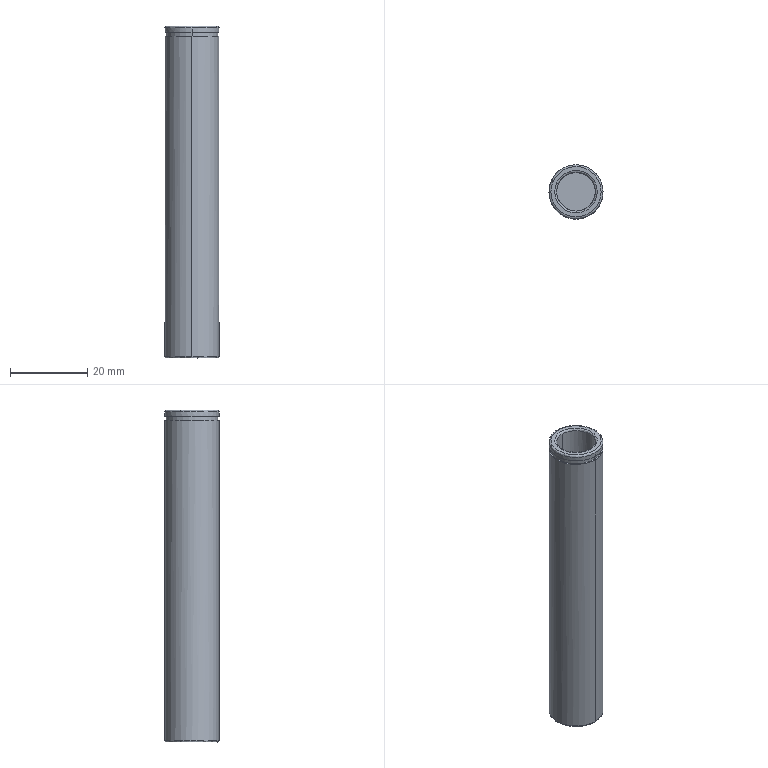Part | SolidWorks | features BaseBody 1 | 1 solid | 30 faces | box 14 x 14 x 86 mm | volume 10942 mm3 | cylinder 14 | spline 8 | plane 8 | commonest cylinder face diameters 10 x4 14 x4 4.2 x2 11.1 x2 13.4 x2
STEP:
#1=CARTESIAN_POINT('',(564.458,-176.727,213.045));
#2=VERTEX_POINT('',#1);
#3=CARTESIAN_POINT('',(552.284,-171.126,213.045));
#4=VERTEX_POINT('',#3);
#5=CARTESIAN_POINT('',(564.458,-176.727,213.045));
#6=CARTESIAN_POINT('',(570.058,-164.553,213.045));
#7=CARTESIAN_POINT('',(557.885,-158.953,213.045));
#8=CARTESIAN_POINT('',(552.284,-171.126,213.045));
#9=(BOUNDED_CURVE()B_SPLINE_CURVE(3,(#5,#6,#7,#8),.UNSPECIFIED.,.F.,.F.)B_SPLINE_CURVE_WITH_KNOTS((4,4),(0.,1.),.UNSPECIFIED.)CURVE()GEOMETRIC_REPRESENTATION_ITEM()RATIONAL_B_SPLINE_CURVE((1.,0.3333,0.3333,1.))REPRESENTATION_ITEM(''));
#10=EDGE_CURVE('',#2,#4,#9,.T.);
#11=ORIENTED_EDGE('',*,*,#10,.T.);
#12=CARTESIAN_POINT('',(552.012,-171.001,213.345));
#13=VERTEX_POINT('',#12);
#14=CARTESIAN_POINT('',(552.284,-171.126,213.345));
#15=DIRECTION('',(0.4179,0.9085,0.000000003));
#16=DIRECTION('',(-0.9085,0.4179,0.000000002));
#17=AXIS2_PLACEMENT_3D('',#14,#15,#16);
#18=CIRCLE('',#17,0.3);
#19=EDGE_CURVE('',#4,#13,#18,.T.);
#20=ORIENTED_EDGE('',*,*,#19,.T.);
#21=CARTESIAN_POINT('',(558.371,-166.927,213.345));
#22=VERTEX_POINT('',#21);
#23=CARTESIAN_POINT('',(558.371,-173.927,213.345));
#24=DIRECTION('',(0.000000001,-0.000000003,1.));
#25=DIRECTION('',(0.,1.,0.000000003));
#26=AXIS2_PLACEMENT_3D('',#23,#24,#25);
#27=CIRCLE('',#26,7.);
#28=EDGE_CURVE('',#22,#13,#27,.T.);
#29=ORIENTED_EDGE('',*,*,#28,.F.);
#30=CARTESIAN_POINT('',(564.73,-176.852,213.345));
#31=VERTEX_POINT('',#30);
#32=CARTESIAN_POINT('',(558.371,-173.927,213.345));
#33=DIRECTION('',(0.000000001,-0.000000003,1.));
#34=DIRECTION('',(0.,1.,0.000000003));
#35=AXIS2_PLACEMENT_3D('',#32,#33,#34);
#36=CIRCLE('',#35,7.);
#37=EDGE_CURVE('',#31,#22,#36,.T.);
#38=ORIENTED_EDGE('',*,*,#37,.F.);
#39=CARTESIAN_POINT('',(564.458,-176.727,213.345));
#40=DIRECTION('',(-0.4179,-0.9085,-0.000000003));
#41=DIRECTION('',(0.9085,-0.4179,-0.000000002));
#42=AXIS2_PLACEMENT_3D('',#39,#40,#41);
#43=CIRCLE('',#42,0.3);
#44=EDGE_CURVE('',#2,#31,#43,.T.);
#45=ORIENTED_EDGE('',*,*,#44,.F.);
#46=EDGE_LOOP('',(#11,#20,#29,#38,#45));
#47=FACE_OUTER_BOUND('',#46,.T.);
#48=CARTESIAN_POINT('',(552.284,-171.126,213.045));
#49=CARTESIAN_POINT('',(557.885,-158.953,213.045));
#50=CARTESIAN_POINT('',(570.058,-164.553,213.045));
#51=CARTESIAN_POINT('',(564.458,-176.727,213.045));
#52=CARTESIAN_POINT('',(552.125,-171.053,213.045));
#53=CARTESIAN_POINT('',(557.872,-158.56,213.045));
#54=CARTESIAN_POINT('',(570.365,-164.307,213.045));
#55=CARTESIAN_POINT('',(564.617,-176.8,213.045));
#56=CARTESIAN_POINT('',(552.012,-171.001,213.169));
#57=CARTESIAN_POINT('',(557.863,-158.282,213.169));
#58=CARTESIAN_POINT('',(570.581,-164.134,213.169));
#59=CARTESIAN_POINT('',(564.73,-176.852,213.169));
#60=CARTESIAN_POINT('',(552.012,-171.001,213.345));
#61=CARTESIAN_POINT('',(557.863,-158.282,213.345));
#62=CARTESIAN_POINT('',(570.581,-164.134,213.345));
#63=CARTESIAN_POINT('',(564.73,-176.852,213.345));
#64=(BOUNDED_SURFACE()B_SPLINE_SURFACE(3,3,((#48,#49,#50,#51),(#52,#53,#54,#55),(#56,#57,#58,#59),(#60,#61,#62,#63)),.UNSPECIFIED.,.F.,.F.,.F.)B_SPLINE_SURFACE_WITH_KNOTS((4,4),(4,4),(0.,1.),(0.,1.),.UNSPECIFIED.)GEOMETRIC_REPRESENTATION_ITEM()RATIONAL_B_SPLINE_SURFACE(((1.,0.3333,0.3333,1.),(0.8047,0.2682,0.2682,0.8047),(0.8047,0.2682,0.2682,0.8047),(1.,0.3333,0.3333,1.)))REPRESENTATION_ITEM('')SURFACE());
#65=ADVANCED_FACE('',(#47),#64,.T.);
#66=CARTESIAN_POINT('',(558.371,-176.027,213.345));
#67=VERTEX_POINT('',#66);
#68=CARTESIAN_POINT('',(560.279,-174.804,213.345));
#69=VERTEX_POINT('',#68);
#70=CARTESIAN_POINT('',(558.371,-173.927,213.345));
#71=DIRECTION('',(0.000000001,-0.000000003,1.));
#72=DIRECTION('',(-0.9085,0.4179,0.000000002));
#73=AXIS2_PLACEMENT_3D('',#70,#71,#72);
#74=CIRCLE('',#73,2.1);
#75=EDGE_CURVE('',#67,#69,#74,.T.);
#76=ORIENTED_EDGE('',*,*,#75,.T.);
#77=CARTESIAN_POINT('',(560.551,-174.93,213.045));
#78=VERTEX_POINT('',#77);
#79=CARTESIAN_POINT('',(560.551,-174.93,213.345));
#80=DIRECTION('',(-0.4179,-0.9085,-0.000000003));
#81=DIRECTION('',(0.9085,-0.4179,-0.000000002));
#82=AXIS2_PLACEMENT_3D('',#79,#80,#81);
#83=CIRCLE('',#82,0.3);
#84=EDGE_CURVE('',#69,#78,#83,.T.);
#85=ORIENTED_EDGE('',*,*,#84,.T.);
#86=CARTESIAN_POINT('',(556.191,-172.924,213.045));
#87=VERTEX_POINT('',#86);
#88=CARTESIAN_POINT('',(556.191,-172.924,213.045));
#89=CARTESIAN_POINT('',(556.127,-173.062,213.045));
#90=CARTESIAN_POINT('',(556.052,-173.275,213.045));
#91=CARTESIAN_POINT('',(556.001,-173.533,213.045));
#92=CARTESIAN_POINT('',(555.985,-173.664,213.045));
#93=CARTESIAN_POINT('',(555.98,-173.721,213.045));
#94=CARTESIAN_POINT('',(555.977,-173.758,213.045));
#95=CARTESIAN_POINT('',(555.976,-173.776,213.045));
#96=CARTESIAN_POINT('',(555.957,-174.127,213.045));
#97=CARTESIAN_POINT('',(556.005,-174.449,213.045));
#98=CARTESIAN_POINT('',(556.177,-174.914,213.045));
#99=CARTESIAN_POINT('',(556.285,-175.134,213.045));
#100=CARTESIAN_POINT('',(556.448,-175.367,213.045));
#101=CARTESIAN_POINT('',(556.539,-175.478,213.045));
#102=CARTESIAN_POINT('',(556.58,-175.524,213.045));
#103=CARTESIAN_POINT('',(556.607,-175.554,213.045));
#104=CARTESIAN_POINT('',(556.623,-175.571,213.045));
#105=CARTESIAN_POINT('',(556.846,-175.805,213.045));
#106=CARTESIAN_POINT('',(557.091,-175.979,213.045));
#107=CARTESIAN_POINT('',(557.506,-176.171,213.045));
#108=CARTESIAN_POINT('',(557.719,-176.245,213.045));
#109=CARTESIAN_POINT('',(557.977,-176.296,213.045));
#110=CARTESIAN_POINT('',(558.108,-176.313,213.045));
#111=CARTESIAN_POINT('',(558.165,-176.318,213.045));
#112=CARTESIAN_POINT('',(558.203,-176.321,213.045));
#113=CARTESIAN_POINT('',(558.22,-176.322,213.045));
#114=CARTESIAN_POINT('',(558.571,-176.341,213.045));
#115=CARTESIAN_POINT('',(558.893,-176.292,213.045));
#116=CARTESIAN_POINT('',(559.359,-176.12,213.045));
#117=CARTESIAN_POINT('',(559.578,-176.013,213.045));
#118=CARTESIAN_POINT('',(559.811,-175.85,213.045));
#119=CARTESIAN_POINT('',(559.922,-175.759,213.045));
#120=CARTESIAN_POINT('',(559.968,-175.718,213.045));
#121=CARTESIAN_POINT('',(559.999,-175.69,213.045));
#122=CARTESIAN_POINT('',(560.015,-175.675,213.045));
#123=CARTESIAN_POINT('',(560.25,-175.451,213.045));
#124=CARTESIAN_POINT('',(560.424,-175.207,213.045));
#125=CARTESIAN_POINT('',(560.551,-174.93,213.045));
#126=B_SPLINE_CURVE_WITH_KNOTS('',3,(#88,#89,#90,#91,#92,#93,#94,#95,#96,#97,#98,#99,#100,#101,#102,#103,#104,#105,#106,#107,#108,#109,#110,#111,#112,#113,#114,#115,#116,#117,#118,#119,#120,#121,#122,#123,#124,#125),.UNSPECIFIED.,.F.,.F.,(4,1,1,1,2,2,2,1,1,1,2,2,2,1,1,1,2,2,2,1,1,1,2,2,4),(0.,0.0625,0.09375,0.1094,0.1172,0.125,0.25,0.3125,0.3437,0.3594,0.3672,0.375,0.5,0.5625,0.5937,0.6094,0.6172,0.625,0.75,0.8125,0.8437,0.8594,0.8672,0.875,1.),.UNSPECIFIED.);
#127=EDGE_CURVE('',#87,#78,#126,.T.);
#128=ORIENTED_EDGE('',*,*,#127,.F.);
#129=CARTESIAN_POINT('',(556.463,-173.049,213.345));
#130=VERTEX_POINT('',#129);
#131=CARTESIAN_POINT('',(556.191,-172.924,213.345));
#132=DIRECTION('',(0.4179,0.9085,0.000000003));
#133=DIRECTION('',(-0.9085,0.4179,0.000000002));
#134=AXIS2_PLACEMENT_3D('',#131,#132,#133);
#135=CIRCLE('',#134,0.3);
#136=EDGE_CURVE('',#130,#87,#135,.T.);
#137=ORIENTED_EDGE('',*,*,#136,.F.);
#138=CARTESIAN_POINT('',(558.371,-173.927,213.345));
#139=DIRECTION('',(0.000000001,-0.000000003,1.));
#140=DIRECTION('',(-0.9085,0.4179,0.000000002));
#141=AXIS2_PLACEMENT_3D('',#138,#139,#140);
#142=CIRCLE('',#141,2.1);
#143=EDGE_CURVE('',#130,#67,#142,.T.);
#144=ORIENTED_EDGE('',*,*,#143,.T.);
#145=EDGE_LOOP('',(#76,#85,#128,#137,#144));
#146=FACE_OUTER_BOUND('',#145,.T.);
#147=CARTESIAN_POINT('',(560.279,-174.804,213.345));
#148=CARTESIAN_POINT('',(558.523,-178.62,213.345));
#149=CARTESIAN_POINT('',(554.708,-176.864,213.345));
#150=CARTESIAN_POINT('',(556.463,-173.049,213.345));
#151=CARTESIAN_POINT('',(560.279,-174.804,213.169));
#152=CARTESIAN_POINT('',(558.523,-178.62,213.169));
#153=CARTESIAN_POINT('',(554.708,-176.864,213.169));
#154=CARTESIAN_POINT('',(556.463,-173.049,213.169));
#155=CARTESIAN_POINT('',(560.392,-174.856,213.045));
#156=CARTESIAN_POINT('',(558.532,-178.898,213.045));
#157=CARTESIAN_POINT('',(554.491,-177.038,213.045));
#158=CARTESIAN_POINT('',(556.35,-172.997,213.045));
#159=CARTESIAN_POINT('',(560.551,-174.93,213.045));
#160=CARTESIAN_POINT('',(558.545,-179.29,213.045));
#161=CARTESIAN_POINT('',(554.185,-177.284,213.045));
#162=CARTESIAN_POINT('',(556.191,-172.924,213.045));
#163=(BOUNDED_SURFACE()B_SPLINE_SURFACE(3,3,((#147,#148,#149,#150),(#151,#152,#153,#154),(#155,#156,#157,#158),(#159,#160,#161,#162)),.UNSPECIFIED.,.F.,.F.,.F.)B_SPLINE_SURFACE_WITH_KNOTS((4,4),(4,4),(0.,1.),(0.,1.),.UNSPECIFIED.)GEOMETRIC_REPRESENTATION_ITEM()RATIONAL_B_SPLINE_SURFACE(((1.,0.3333,0.3333,1.),(0.8047,0.2682,0.2682,0.8047),(0.8047,0.2682,0.2682,0.8047),(1.,0.3333,0.3333,1.)))REPRESENTATION_ITEM('')SURFACE());
#164=ADVANCED_FACE('',(#146),#163,.T.);
#165=CARTESIAN_POINT('',(564.276,-176.643,299.045));
#166=VERTEX_POINT('',#165);
#167=CARTESIAN_POINT('',(552.466,-171.21,299.045));
#168=VERTEX_POINT('',#167);
#169=CARTESIAN_POINT('',(564.276,-176.643,299.045));
#170=CARTESIAN_POINT('',(558.843,-188.453,299.045));
#171=CARTESIAN_POINT('',(547.033,-183.02,299.045));
#172=CARTESIAN_POINT('',(552.466,-171.21,299.045));
#173=(BOUNDED_CURVE()B_SPLINE_CURVE(3,(#169,#170,#171,#172),.UNSPECIFIED.,.F.,.F.)B_SPLINE_CURVE_WITH_KNOTS((4,4),(0.,1.),.UNSPECIFIED.)CURVE()GEOMETRIC_REPRESENTATION_ITEM()RATIONAL_B_SPLINE_CURVE((1.,0.3333,0.3333,1.))REPRESENTATION_ITEM(''));
#174=EDGE_CURVE('',#166,#168,#173,.T.);
#175=ORIENTED_EDGE('',*,*,#174,.T.);
#176=CARTESIAN_POINT('',(552.012,-171.001,298.545));
#177=VERTEX_POINT('',#176);
#178=CARTESIAN_POINT('',(552.466,-171.21,298.545));
#179=DIRECTION('',(-0.4179,-0.9085,-0.000000003));
#180=DIRECTION('',(-0.9085,0.4179,0.000000002));
#181=AXIS2_PLACEMENT_3D('',#178,#179,#180);
#182=CIRCLE('',#181,0.5);
#183=EDGE_CURVE('',#168,#177,#182,.T.);
#184=ORIENTED_EDGE('',*,*,#183,.T.);
#185=CARTESIAN_POINT('',(558.371,-180.927,298.545));
#186=VERTEX_POINT('',#185);
#187=CARTESIAN_POINT('',(558.371,-173.927,298.545));
#188=DIRECTION('',(-0.000000001,0.000000003,-1.));
#189=DIRECTION('',(0.,1.,0.000000003));
#190=AXIS2_PLACEMENT_3D('',#187,#188,#189);
#191=CIRCLE('',#190,7.);
#192=EDGE_CURVE('',#186,#177,#191,.T.);
#193=ORIENTED_EDGE('',*,*,#192,.F.);
#194=CARTESIAN_POINT('',(564.73,-176.852,298.545));
#195=VERTEX_POINT('',#194);
#196=CARTESIAN_POINT('',(558.371,-173.927,298.545));
#197=DIRECTION('',(-0.000000001,0.000000003,-1.));
#198=DIRECTION('',(0.,1.,0.000000003));
#199=AXIS2_PLACEMENT_3D('',#196,#197,#198);
#200=CIRCLE('',#199,7.);
#201=EDGE_CURVE('',#195,#186,#200,.T.);
#202=ORIENTED_EDGE('',*,*,#201,.F.);
#203=CARTESIAN_POINT('',(564.276,-176.643,298.545));
#204=DIRECTION('',(0.4179,0.9085,0.000000003));
#205=DIRECTION('',(0.9085,-0.4179,-0.000000002));
#206=AXIS2_PLACEMENT_3D('',#203,#204,#205);
#207=CIRCLE('',#206,0.5);
#208=EDGE_CURVE('',#166,#195,#207,.T.);
#209=ORIENTED_EDGE('',*,*,#208,.F.);
#210=EDGE_LOOP('',(#175,#184,#193,#202,#209));
#211=FACE_OUTER_BOUND('',#210,.T.);
#212=CARTESIAN_POINT('',(552.466,-171.21,299.045));
#213=CARTESIAN_POINT('',(547.033,-183.02,299.045));
#214=CARTESIAN_POINT('',(558.843,-188.453,299.045));
#215=CARTESIAN_POINT('',(564.276,-176.643,299.045));
#216=CARTESIAN_POINT('',(552.2,-171.088,299.045));
#217=CARTESIAN_POINT('',(546.522,-183.43,299.045));
#218=CARTESIAN_POINT('',(558.864,-189.108,299.045));
#219=CARTESIAN_POINT('',(564.542,-176.766,299.045));
#220=CARTESIAN_POINT('',(552.012,-171.001,298.837));
#221=CARTESIAN_POINT('',(546.161,-183.72,298.837));
#222=CARTESIAN_POINT('',(558.879,-189.571,298.837));
#223=CARTESIAN_POINT('',(564.73,-176.852,298.837));
#224=CARTESIAN_POINT('',(552.012,-171.001,298.545));
#225=CARTESIAN_POINT('',(546.161,-183.72,298.545));
#226=CARTESIAN_POINT('',(558.879,-189.571,298.545));
#227=CARTESIAN_POINT('',(564.73,-176.852,298.545));
#228=(BOUNDED_SURFACE()B_SPLINE_SURFACE(3,3,((#212,#213,#214,#215),(#216,#217,#218,#219),(#220,#221,#222,#223),(#224,#225,#226,#227)),.UNSPECIFIED.,.F.,.F.,.F.)B_SPLINE_SURFACE_WITH_KNOTS((4,4),(4,4),(0.,1.),(0.,1.),.UNSPECIFIED.)GEOMETRIC_REPRESENTATION_ITEM()RATIONAL_B_SPLINE_SURFACE(((1.,0.3333,0.3333,1.),(0.8047,0.2682,0.2682,0.8047),(0.8047,0.2682,0.2682,0.8047),(1.,0.3333,0.3333,1.)))REPRESENTATION_ITEM('')SURFACE());
#229=ADVANCED_FACE('',(#211),#228,.T.);
#230=CARTESIAN_POINT('',(558.371,-178.927,298.545));
#231=VERTEX_POINT('',#230);
#232=CARTESIAN_POINT('',(553.829,-171.837,298.545));
#233=VERTEX_POINT('',#232);
#234=CARTESIAN_POINT('',(558.371,-173.927,298.545));
#235=DIRECTION('',(-0.000000001,0.000000003,-1.));
#236=DIRECTION('',(0.9085,-0.4179,-0.000000002));
#237=AXIS2_PLACEMENT_3D('',#234,#235,#236);
#238=CIRCLE('',#237,5.);
#239=EDGE_CURVE('',#231,#233,#238,.T.);
#240=ORIENTED_EDGE('',*,*,#239,.T.);
#241=CARTESIAN_POINT('',(553.374,-171.628,299.045));
#242=VERTEX_POINT('',#241);
#243=CARTESIAN_POINT('',(553.374,-171.628,298.545));
#244=DIRECTION('',(-0.4179,-0.9085,-0.000000003));
#245=DIRECTION('',(-0.9085,0.4179,0.000000002));
#246=AXIS2_PLACEMENT_3D('',#243,#244,#245);
#247=CIRCLE('',#246,0.5);
#248=EDGE_CURVE('',#233,#242,#247,.T.);
#249=ORIENTED_EDGE('',*,*,#248,.T.);
#250=CARTESIAN_POINT('',(563.368,-176.225,299.045));
#251=VERTEX_POINT('',#250);
#252=CARTESIAN_POINT('',(553.374,-171.628,299.045));
#253=CARTESIAN_POINT('',(548.777,-181.621,299.045));
#254=CARTESIAN_POINT('',(558.77,-186.218,299.045));
#255=CARTESIAN_POINT('',(563.368,-176.225,299.045));
#256=(BOUNDED_CURVE()B_SPLINE_CURVE(3,(#252,#253,#254,#255),.UNSPECIFIED.,.F.,.F.)B_SPLINE_CURVE_WITH_KNOTS((4,4),(0.,1.),.UNSPECIFIED.)CURVE()GEOMETRIC_REPRESENTATION_ITEM()RATIONAL_B_SPLINE_CURVE((1.,0.3333,0.3333,1.))REPRESENTATION_ITEM(''));
#257=EDGE_CURVE('',#242,#251,#256,.T.);
#258=ORIENTED_EDGE('',*,*,#257,.T.);
#259=CARTESIAN_POINT('',(562.913,-176.016,298.545));
#260=VERTEX_POINT('',#259);
#261=CARTESIAN_POINT('',(563.368,-176.225,298.545));
#262=DIRECTION('',(0.4179,0.9085,0.000000003));
#263=DIRECTION('',(0.9085,-0.4179,-0.000000002));
#264=AXIS2_PLACEMENT_3D('',#261,#262,#263);
#265=CIRCLE('',#264,0.5);
#266=EDGE_CURVE('',#260,#251,#265,.T.);
#267=ORIENTED_EDGE('',*,*,#266,.F.);
#268=CARTESIAN_POINT('',(558.371,-173.927,298.545));
#269=DIRECTION('',(-0.000000001,0.000000003,-1.));
#270=DIRECTION('',(0.9085,-0.4179,-0.000000002));
#271=AXIS2_PLACEMENT_3D('',#268,#269,#270);
#272=CIRCLE('',#271,5.);
#273=EDGE_CURVE('',#260,#231,#272,.T.);
#274=ORIENTED_EDGE('',*,*,#273,.T.);
#275=EDGE_LOOP('',(#240,#249,#258,#267,#274));
#276=FACE_OUTER_BOUND('',#275,.T.);
#277=CARTESIAN_POINT('',(553.829,-171.837,298.545));
#278=CARTESIAN_POINT('',(549.649,-180.922,298.545));
#279=CARTESIAN_POINT('',(558.734,-185.101,298.545));
#280=CARTESIAN_POINT('',(562.913,-176.016,298.545));
#281=CARTESIAN_POINT('',(553.829,-171.837,298.837));
#282=CARTESIAN_POINT('',(549.649,-180.922,298.837));
#283=CARTESIAN_POINT('',(558.734,-185.101,298.837));
#284=CARTESIAN_POINT('',(562.913,-176.016,298.837));
#285=CARTESIAN_POINT('',(553.64,-171.75,299.045));
#286=CARTESIAN_POINT('',(549.288,-181.211,299.045));
#287=CARTESIAN_POINT('',(558.749,-185.564,299.045));
#288=CARTESIAN_POINT('',(563.102,-176.103,299.045));
#289=CARTESIAN_POINT('',(553.374,-171.628,299.045));
#290=CARTESIAN_POINT('',(548.777,-181.621,299.045));
#291=CARTESIAN_POINT('',(558.77,-186.218,299.045));
#292=CARTESIAN_POINT('',(563.368,-176.225,299.045));
#293=(BOUNDED_SURFACE()B_SPLINE_SURFACE(3,3,((#277,#278,#279,#280),(#281,#282,#283,#284),(#285,#286,#287,#288),(#289,#290,#291,#292)),.UNSPECIFIED.,.F.,.F.,.F.)B_SPLINE_SURFACE_WITH_KNOTS((4,4),(4,4),(0.,1.),(0.,1.),.UNSPECIFIED.)GEOMETRIC_REPRESENTATION_ITEM()RATIONAL_B_SPLINE_SURFACE(((1.,0.3333,0.3333,1.),(0.8047,0.2682,0.2682,0.8047),(0.8047,0.2682,0.2682,0.8047),(1.,0.3333,0.3333,1.)))REPRESENTATION_ITEM('')SURFACE());
#294=ADVANCED_FACE('',(#276),#293,.T.);
#295=CARTESIAN_POINT('',(558.371,-166.927,296.336));
#296=VERTEX_POINT('',#295);
#297=CARTESIAN_POINT('',(558.371,-180.927,296.336));
#298=VERTEX_POINT('',#297);
#299=CARTESIAN_POINT('',(558.371,-173.927,296.336));
#300=DIRECTION('',(-0.000000001,0.000000003,-1.));
#301=DIRECTION('',(0.,1.,0.000000003));
#302=AXIS2_PLACEMENT_3D('',#299,#300,#301);
#303=CIRCLE('',#302,7.);
#304=EDGE_CURVE('',#296,#298,#303,.T.);
#305=ORIENTED_EDGE('',*,*,#304,.T.);
#306=CARTESIAN_POINT('',(558.371,-180.927,213.345));
#307=VERTEX_POINT('',#306);
#308=CARTESIAN_POINT('',(558.371,-180.927,299.045));
#309=DIRECTION('',(-0.000000001,0.000000003,-1.));
#310=VECTOR('',#309,1000.);
#311=LINE('',#308,#310);
#312=EDGE_CURVE('',#298,#307,#311,.T.);
#313=ORIENTED_EDGE('',*,*,#312,.T.);
#314=CARTESIAN_POINT('',(558.371,-173.927,213.345));
#315=DIRECTION('',(0.000000001,-0.000000003,1.));
#316=DIRECTION('',(0.,1.,0.000000003));
#317=AXIS2_PLACEMENT_3D('',#314,#315,#316);
#318=CIRCLE('',#317,7.);
#319=EDGE_CURVE('',#307,#31,#318,.T.);
#320=ORIENTED_EDGE('',*,*,#319,.T.);
#321=ORIENTED_EDGE('',*,*,#37,.T.);
#322=CARTESIAN_POINT('',(558.371,-166.927,299.045));
#323=DIRECTION('',(-0.000000001,0.000000003,-1.));
#324=VECTOR('',#323,1000.);
#325=LINE('',#322,#324);
#326=EDGE_CURVE('',#296,#22,#325,.T.);
#327=ORIENTED_EDGE('',*,*,#326,.F.);
#328=EDGE_LOOP('',(#305,#313,#320,#321,#327));
#329=FACE_OUTER_BOUND('',#328,.T.);
#330=CARTESIAN_POINT('',(558.371,-173.927,299.045));
#331=DIRECTION('',(-0.000000001,0.000000003,-1.));
#332=DIRECTION('',(0.,1.,0.000000003));
#333=AXIS2_PLACEMENT_3D('',#330,#331,#332);
#334=CYLINDRICAL_SURFACE('',#333,7.);
#335=ADVANCED_FACE('',(#329),#334,.T.);
#336=CARTESIAN_POINT('',(558.371,-180.627,296.336));
#337=VERTEX_POINT('',#336);
#338=CARTESIAN_POINT('',(558.371,-167.227,296.336));
#339=VERTEX_POINT('',#338);
#340=CARTESIAN_POINT('',(558.371,-173.927,296.336));
#341=DIRECTION('',(0.000000001,-0.000000003,1.));
#342=DIRECTION('',(0.,-1.,-0.000000003));
#343=AXIS2_PLACEMENT_3D('',#340,#341,#342);
#344=CIRCLE('',#343,6.7);
#345=EDGE_CURVE('',#337,#339,#344,.T.);
#346=ORIENTED_EDGE('',*,*,#345,.T.);
#347=CARTESIAN_POINT('',(558.371,-167.227,297.436));
#348=VERTEX_POINT('',#347);
#349=CARTESIAN_POINT('',(558.371,-167.227,296.886));
#350=DIRECTION('',(0.000000001,-0.000000003,1.));
#351=VECTOR('',#350,1000.);
#352=LINE('',#349,#351);
#353=EDGE_CURVE('',#339,#348,#352,.T.);
#354=ORIENTED_EDGE('',*,*,#353,.T.);
#355=CARTESIAN_POINT('',(558.371,-180.627,297.436));
#356=VERTEX_POINT('',#355);
#357=CARTESIAN_POINT('',(558.371,-173.927,297.436));
#358=DIRECTION('',(-0.000000001,0.000000003,-1.));
#359=DIRECTION('',(0.,-1.,-0.000000003));
#360=AXIS2_PLACEMENT_3D('',#357,#358,#359);
#361=CIRCLE('',#360,6.7);
#362=EDGE_CURVE('',#348,#356,#361,.T.);
#363=ORIENTED_EDGE('',*,*,#362,.T.);
#364=CARTESIAN_POINT('',(558.371,-180.627,296.886));
#365=DIRECTION('',(0.000000001,-0.000000003,1.));
#366=VECTOR('',#365,1000.);
#367=LINE('',#364,#366);
#368=EDGE_CURVE('',#337,#356,#367,.T.);
#369=ORIENTED_EDGE('',*,*,#368,.F.);
#370=EDGE_LOOP('',(#346,#354,#363,#369));
#371=FACE_OUTER_BOUND('',#370,.T.);
#372=CARTESIAN_POINT('',(558.371,-173.927,296.886));
#373=DIRECTION('',(0.000000001,-0.000000003,1.));
#374=DIRECTION('',(0.,-1.,-0.000000003));
#375=AXIS2_PLACEMENT_3D('',#372,#373,#374);
#376=CYLINDRICAL_SURFACE('',#375,6.7);
#377=ADVANCED_FACE('',(#371),#376,.T.);
#378=CARTESIAN_POINT('',(558.371,-176.027,229.045));
#379=VERTEX_POINT('',#378);
#380=CARTESIAN_POINT('',(558.371,-171.827,229.045));
#381=VERTEX_POINT('',#380);
#382=CARTESIAN_POINT('',(558.371,-173.927,229.045));
#383=DIRECTION('',(-0.000000001,0.000000003,-1.));
#384=DIRECTION('',(0.,1.,0.000000003));
#385=AXIS2_PLACEMENT_3D('',#382,#383,#384);
#386=CIRCLE('',#385,2.1);
#387=EDGE_CURVE('',#379,#381,#386,.T.);
#388=ORIENTED_EDGE('',*,*,#387,.F.);
#389=CARTESIAN_POINT('',(558.371,-176.027,221.045));
#390=DIRECTION('',(-0.000000001,0.000000003,-1.));
#391=VECTOR('',#390,1000.);
#392=LINE('',#389,#391);
#393=EDGE_CURVE('',#379,#67,#392,.T.);
#394=ORIENTED_EDGE('',*,*,#393,.T.);
#395=ORIENTED_EDGE('',*,*,#143,.F.);
#396=CARTESIAN_POINT('',(558.371,-171.827,213.345));
#397=VERTEX_POINT('',#396);
#398=CARTESIAN_POINT('',(558.371,-173.927,213.345));
#399=DIRECTION('',(0.000000001,-0.000000003,1.));
#400=DIRECTION('',(-0.9085,0.4179,0.000000002));
#401=AXIS2_PLACEMENT_3D('',#398,#399,#400);
#402=CIRCLE('',#401,2.1);
#403=EDGE_CURVE('',#397,#130,#402,.T.);
#404=ORIENTED_EDGE('',*,*,#403,.F.);
#405=CARTESIAN_POINT('',(558.371,-171.827,221.045));
#406=DIRECTION('',(-0.000000001,0.000000003,-1.));
#407=VECTOR('',#406,1000.);
#408=LINE('',#405,#407);
#409=EDGE_CURVE('',#381,#397,#408,.T.);
#410=ORIENTED_EDGE('',*,*,#409,.F.);
#411=EDGE_LOOP('',(#388,#394,#395,#404,#410));
#412=FACE_OUTER_BOUND('',#411,.T.);
#413=CARTESIAN_POINT('',(558.371,-173.927,221.045));
#414=DIRECTION('',(-0.000000001,0.000000003,-1.));
#415=DIRECTION('',(0.,1.,0.000000003));
#416=AXIS2_PLACEMENT_3D('',#413,#414,#415);
#417=CYLINDRICAL_SURFACE('',#416,2.1);
#418=ADVANCED_FACE('',(#412),#417,.F.);
#419=CARTESIAN_POINT('',(558.371,-166.927,298.545));
#420=VERTEX_POINT('',#419);
#421=CARTESIAN_POINT('',(558.371,-173.927,298.545));
#422=DIRECTION('',(-0.000000001,0.000000003,-1.));
#423=DIRECTION('',(0.,1.,0.000000003));
#424=AXIS2_PLACEMENT_3D('',#421,#422,#423);
#425=CIRCLE('',#424,7.);
#426=EDGE_CURVE('',#420,#195,#425,.T.);
#427=ORIENTED_EDGE('',*,*,#426,.T.);
#428=ORIENTED_EDGE('',*,*,#201,.T.);
#429=CARTESIAN_POINT('',(558.371,-180.927,297.436));
#430=VERTEX_POINT('',#429);
#431=CARTESIAN_POINT('',(558.371,-180.927,299.045));
#432=DIRECTION('',(-0.000000001,0.000000003,-1.));
#433=VECTOR('',#432,1000.);
#434=LINE('',#431,#433);
#435=EDGE_CURVE('',#186,#430,#434,.T.);
#436=ORIENTED_EDGE('',*,*,#435,.T.);
#437=CARTESIAN_POINT('',(558.371,-166.927,297.436));
#438=VERTEX_POINT('',#437);
#439=CARTESIAN_POINT('',(558.371,-173.927,297.436));
#440=DIRECTION('',(0.000000001,-0.000000003,1.));
#441=DIRECTION('',(0.,1.,0.000000003));
#442=AXIS2_PLACEMENT_3D('',#439,#440,#441);
#443=CIRCLE('',#442,7.);
#444=EDGE_CURVE('',#430,#438,#443,.T.);
#445=ORIENTED_EDGE('',*,*,#444,.T.);
#446=CARTESIAN_POINT('',(558.371,-166.927,299.045));
#447=DIRECTION('',(-0.000000001,0.000000003,-1.));
#448=VECTOR('',#447,1000.);
#449=LINE('',#446,#448);
#450=EDGE_CURVE('',#420,#438,#449,.T.);
#451=ORIENTED_EDGE('',*,*,#450,.F.);
#452=EDGE_LOOP('',(#427,#428,#436,#445,#451));
#453=FACE_OUTER_BOUND('',#452,.T.);
#454=CARTESIAN_POINT('',(558.371,-173.927,299.045));
#455=DIRECTION('',(-0.000000001,0.000000003,-1.));
#456=DIRECTION('',(0.,1.,0.000000003));
#457=AXIS2_PLACEMENT_3D('',#454,#455,#456);
#458=CYLINDRICAL_SURFACE('',#457,7.);
#459=ADVANCED_FACE('',(#453),#458,.T.);
#460=ORIENTED_EDGE('',*,*,#239,.F.);
#461=CARTESIAN_POINT('',(558.371,-178.927,283.745));
#462=VERTEX_POINT('',#461);
#463=CARTESIAN_POINT('',(558.371,-178.927,299.045));
#464=DIRECTION('',(-0.000000001,0.000000003,-1.));
#465=VECTOR('',#464,1000.);
#466=LINE('',#463,#465);
#467=EDGE_CURVE('',#231,#462,#466,.T.);
#468=ORIENTED_EDGE('',*,*,#467,.T.);
#469=CARTESIAN_POINT('',(558.371,-168.927,283.745));
#470=VERTEX_POINT('',#469);
#471=CARTESIAN_POINT('',(558.371,-173.927,283.745));
#472=DIRECTION('',(0.000000001,-0.000000003,1.));
#473=DIRECTION('',(0.,1.,0.000000003));
#474=AXIS2_PLACEMENT_3D('',#471,#472,#473);
#475=CIRCLE('',#474,5.);
#476=EDGE_CURVE('',#470,#462,#475,.T.);
#477=ORIENTED_EDGE('',*,*,#476,.F.);
#478=CARTESIAN_POINT('',(558.371,-168.927,298.545));
#479=VERTEX_POINT('',#478);
#480=CARTESIAN_POINT('',(558.371,-168.927,299.045));
#481=DIRECTION('',(-0.000000001,0.000000003,-1.));
#482=VECTOR('',#481,1000.);
#483=LINE('',#480,#482);
#484=EDGE_CURVE('',#479,#470,#483,.T.);
#485=ORIENTED_EDGE('',*,*,#484,.F.);
#486=CARTESIAN_POINT('',(558.371,-173.927,298.545));
#487=DIRECTION('',(-0.000000001,0.000000003,-1.));
#488=DIRECTION('',(0.9085,-0.4179,-0.000000002));
#489=AXIS2_PLACEMENT_3D('',#486,#487,#488);
#490=CIRCLE('',#489,5.);
#491=EDGE_CURVE('',#233,#479,#490,.T.);
#492=ORIENTED_EDGE('',*,*,#491,.F.);
#493=EDGE_LOOP('',(#460,#468,#477,#485,#492));
#494=FACE_OUTER_BOUND('',#493,.T.);
#495=CARTESIAN_POINT('',(558.371,-173.927,299.045));
#496=DIRECTION('',(-0.000000001,0.000000003,-1.));
#497=DIRECTION('',(0.,1.,0.000000003));
#498=AXIS2_PLACEMENT_3D('',#495,#496,#497);
#499=CYLINDRICAL_SURFACE('',#498,5.);
#500=ADVANCED_FACE('',(#494),#499,.F.);
#501=CARTESIAN_POINT('',(558.371,-168.377,283.045));
#502=VERTEX_POINT('',#501);
#503=CARTESIAN_POINT('',(558.371,-179.477,283.045));
#504=VERTEX_POINT('',#503);
#505=CARTESIAN_POINT('',(558.371,-173.927,283.045));
#506=DIRECTION('',(0.000000001,-0.000000003,1.));
#507=DIRECTION('',(0.,-1.,-0.000000003));
#508=AXIS2_PLACEMENT_3D('',#505,#506,#507);
#509=CIRCLE('',#508,5.55);
#510=EDGE_CURVE('',#502,#504,#509,.T.);
#511=ORIENTED_EDGE('',*,*,#510,.F.);
#512=CARTESIAN_POINT('',(558.371,-168.377,283.745));
#513=VERTEX_POINT('',#512);
#514=CARTESIAN_POINT('',(558.371,-168.377,283.745));
#515=DIRECTION('',(0.000000001,-0.000000003,1.));
#516=VECTOR('',#515,1000.);
#517=LINE('',#514,#516);
#518=EDGE_CURVE('',#502,#513,#517,.T.);
#519=ORIENTED_EDGE('',*,*,#518,.T.);
#520=CARTESIAN_POINT('',(558.371,-179.477,283.745));
#521=VERTEX_POINT('',#520);
#522=CARTESIAN_POINT('',(558.371,-173.927,283.745));
#523=DIRECTION('',(-0.000000001,0.000000003,-1.));
#524=DIRECTION('',(0.,-1.,-0.000000003));
#525=AXIS2_PLACEMENT_3D('',#522,#523,#524);
#526=CIRCLE('',#525,5.55);
#527=EDGE_CURVE('',#521,#513,#526,.T.);
#528=ORIENTED_EDGE('',*,*,#527,.F.);
#529=CARTESIAN_POINT('',(558.371,-179.477,283.745));
#530=DIRECTION('',(0.000000001,-0.000000003,1.));
#531=VECTOR('',#530,1000.);
#532=LINE('',#529,#531);
#533=EDGE_CURVE('',#504,#521,#532,.T.);
#534=ORIENTED_EDGE('',*,*,#533,.F.);
#535=EDGE_LOOP('',(#511,#519,#528,#534));
#536=FACE_OUTER_BOUND('',#535,.T.);
#537=CARTESIAN_POINT('',(558.371,-173.927,283.745));
#538=DIRECTION('',(0.000000001,-0.000000003,1.));
#539=DIRECTION('',(0.,-1.,-0.000000003));
#540=AXIS2_PLACEMENT_3D('',#537,#538,#539);
#541=CYLINDRICAL_SURFACE('',#540,5.55);
#542=ADVANCED_FACE('',(#536),#541,.F.);
#543=CARTESIAN_POINT('',(558.371,-168.927,283.045));
#544=VERTEX_POINT('',#543);
#545=CARTESIAN_POINT('',(558.371,-178.927,283.045));
#546=VERTEX_POINT('',#545);
#547=CARTESIAN_POINT('',(558.371,-173.927,283.045));
#548=DIRECTION('',(0.000000001,-0.000000003,1.));
#549=DIRECTION('',(0.,1.,0.000000003));
#550=AXIS2_PLACEMENT_3D('',#547,#548,#549);
#551=CIRCLE('',#550,5.);
#552=EDGE_CURVE('',#544,#546,#551,.T.);
#553=ORIENTED_EDGE('',*,*,#552,.T.);
#554=CARTESIAN_POINT('',(558.371,-178.927,273.045));
#555=VERTEX_POINT('',#554);
#556=CARTESIAN_POINT('',(558.371,-178.927,299.045));
#557=DIRECTION('',(-0.000000001,0.000000003,-1.));
#558=VECTOR('',#557,1000.);
#559=LINE('',#556,#558);
#560=EDGE_CURVE('',#546,#555,#559,.T.);
#561=ORIENTED_EDGE('',*,*,#560,.T.);
#562=CARTESIAN_POINT('',(558.371,-168.927,273.045));
#563=VERTEX_POINT('',#562);
#564=CARTESIAN_POINT('',(558.371,-173.927,273.045));
#565=DIRECTION('',(0.000000001,-0.000000003,1.));
#566=DIRECTION('',(0.,1.,0.000000003));
#567=AXIS2_PLACEMENT_3D('',#564,#565,#566);
#568=CIRCLE('',#567,5.);
#569=EDGE_CURVE('',#563,#555,#568,.T.);
#570=ORIENTED_EDGE('',*,*,#569,.F.);
#571=CARTESIAN_POINT('',(558.371,-168.927,299.045));
#572=DIRECTION('',(-0.000000001,0.000000003,-1.));
#573=VECTOR('',#572,1000.);
#574=LINE('',#571,#573);
#575=EDGE_CURVE('',#544,#563,#574,.T.);
#576=ORIENTED_EDGE('',*,*,#575,.F.);
#577=EDGE_LOOP('',(#553,#561,#570,#576));
#578=FACE_OUTER_BOUND('',#577,.T.);
#579=CARTESIAN_POINT('',(558.371,-173.927,299.045));
#580=DIRECTION('',(-0.000000001,0.000000003,-1.));
#581=DIRECTION('',(0.,1.,0.000000003));
#582=AXIS2_PLACEMENT_3D('',#579,#580,#581);
#583=CYLINDRICAL_SURFACE('',#582,5.);
#584=ADVANCED_FACE('',(#578),#583,.F.);
#585=ORIENTED_EDGE('',*,*,#312,.F.);
#586=CARTESIAN_POINT('',(558.371,-173.927,296.336));
#587=DIRECTION('',(-0.000000001,0.000000003,-1.));
#588=DIRECTION('',(0.,1.,0.000000003));
#589=AXIS2_PLACEMENT_3D('',#586,#587,#588);
#590=CIRCLE('',#589,7.);
#591=EDGE_CURVE('',#298,#296,#590,.T.);
#592=ORIENTED_EDGE('',*,*,#591,.T.);
#593=ORIENTED_EDGE('',*,*,#326,.T.);
#594=ORIENTED_EDGE('',*,*,#28,.T.);
#595=CARTESIAN_POINT('',(558.371,-173.927,213.345));
#596=DIRECTION('',(0.000000001,-0.000000003,1.));
#597=DIRECTION('',(0.,1.,0.000000003));
#598=AXIS2_PLACEMENT_3D('',#595,#596,#597);
#599=CIRCLE('',#598,7.);
#600=EDGE_CURVE('',#13,#307,#599,.T.);
#601=ORIENTED_EDGE('',*,*,#600,.T.);
#602=EDGE_LOOP('',(#585,#592,#593,#594,#601));
#603=FACE_OUTER_BOUND('',#602,.T.);
#604=CARTESIAN_POINT('',(558.371,-173.927,299.045));
#605=DIRECTION('',(-0.000000001,0.000000003,-1.));
#606=DIRECTION('',(0.,1.,0.000000003));
#607=AXIS2_PLACEMENT_3D('',#604,#605,#606);
#608=CYLINDRICAL_SURFACE('',#607,7.);
#609=ADVANCED_FACE('',(#603),#608,.T.);
#610=ORIENTED_EDGE('',*,*,#19,.F.);
#611=CARTESIAN_POINT('',(564.458,-176.727,213.045));
#612=CARTESIAN_POINT('',(564.372,-176.913,213.045));
#613=CARTESIAN_POINT('',(564.232,-177.185,213.045));
#614=CARTESIAN_POINT('',(564.046,-177.49,213.045));
#615=CARTESIAN_POINT('',(563.948,-177.64,213.045));
#616=CARTESIAN_POINT('',(563.905,-177.703,213.045));
#617=CARTESIAN_POINT('',(563.876,-177.746,213.045));
#618=CARTESIAN_POINT('',(563.862,-177.765,213.045));
#619=CARTESIAN_POINT('',(563.722,-177.965,213.045));
#620=CARTESIAN_POINT('',(563.522,-178.221,213.045));
#621=CARTESIAN_POINT('',(563.268,-178.502,213.045));
#622=CARTESIAN_POINT('',(563.154,-178.618,213.045));
#623=CARTESIAN_POINT('',(563.078,-178.695,213.045));
#624=CARTESIAN_POINT('',(563.041,-178.732,213.045));
#625=CARTESIAN_POINT('',(562.836,-178.927,213.045));
#626=CARTESIAN_POINT('',(562.58,-179.148,213.045));
#627=CARTESIAN_POINT('',(562.263,-179.382,213.045));
#628=CARTESIAN_POINT('',(562.123,-179.478,213.045));
#629=CARTESIAN_POINT('',(562.029,-179.54,213.045));
#630=CARTESIAN_POINT('',(561.982,-179.57,213.045));
#631=CARTESIAN_POINT('',(561.542,-179.847,213.045));
#632=CARTESIAN_POINT('',(561.128,-180.05,213.045));
#633=CARTESIAN_POINT('',(560.478,-180.291,213.045));
#634=CARTESIAN_POINT('',(560.149,-180.394,213.045));
#635=CARTESIAN_POINT('',(559.756,-180.484,213.045));
#636=CARTESIAN_POINT('',(559.586,-180.516,213.045));
#637=CARTESIAN_POINT('',(559.472,-180.536,213.045));
#638=CARTESIAN_POINT('',(559.414,-180.545,213.045));
#639=CARTESIAN_POINT('',(559.134,-180.587,213.045));
#640=CARTESIAN_POINT('',(558.798,-180.62,213.045));
#641=CARTESIAN_POINT('',(558.403,-180.628,213.045));
#642=CARTESIAN_POINT('',(558.206,-180.625,213.045));
#643=CARTESIAN_POINT('',(558.121,-180.622,213.045));
#644=CARTESIAN_POINT('',(558.064,-180.62,213.045));
#645=CARTESIAN_POINT('',(558.035,-180.618,213.045));
#646=CARTESIAN_POINT('',(557.791,-180.605,213.045));
#647=CARTESIAN_POINT('',(557.468,-180.572,213.045));
#648=CARTESIAN_POINT('',(557.095,-180.506,213.045));
#649=CARTESIAN_POINT('',(556.91,-180.466,213.045));
#650=CARTESIAN_POINT('',(556.831,-180.447,213.045));
#651=CARTESIAN_POINT('',(556.778,-180.434,213.045));
#652=CARTESIAN_POINT('',(556.75,-180.428,213.045));
#653=CARTESIAN_POINT('',(556.328,-180.321,213.045));
#654=CARTESIAN_POINT('',(555.943,-180.184,213.045));
#655=CARTESIAN_POINT('',(555.385,-179.928,213.045));
#656=CARTESIAN_POINT('',(555.113,-179.787,213.045));
#657=CARTESIAN_POINT('',(554.807,-179.602,213.045));
#658=CARTESIAN_POINT('',(554.658,-179.504,213.045));
#659=CARTESIAN_POINT('',(554.594,-179.461,213.045));
#660=CARTESIAN_POINT('',(554.552,-179.432,213.045));
#661=CARTESIAN_POINT('',(554.532,-179.418,213.045));
#662=CARTESIAN_POINT('',(554.333,-179.277,213.045));
#663=CARTESIAN_POINT('',(554.077,-179.077,213.045));
#664=CARTESIAN_POINT('',(553.796,-178.823,213.045));
#665=CARTESIAN_POINT('',(553.679,-178.71,213.045));
#666=CARTESIAN_POINT('',(553.602,-178.633,213.045));
#667=CARTESIAN_POINT('',(553.566,-178.596,213.045));
#668=CARTESIAN_POINT('',(553.371,-178.392,213.045));
#669=CARTESIAN_POINT('',(553.15,-178.136,213.045));
#670=CARTESIAN_POINT('',(552.915,-177.818,213.045));
#671=CARTESIAN_POINT('',(552.82,-177.679,213.045));
#672=CARTESIAN_POINT('',(552.757,-177.584,213.045));
#673=CARTESIAN_POINT('',(552.727,-177.538,213.045));
#674=CARTESIAN_POINT('',(552.451,-177.097,213.045));
#675=CARTESIAN_POINT('',(552.247,-176.684,213.045));
#676=CARTESIAN_POINT('',(552.007,-176.034,213.045));
#677=CARTESIAN_POINT('',(551.904,-175.704,213.045));
#678=CARTESIAN_POINT('',(551.814,-175.311,213.045));
#679=CARTESIAN_POINT('',(551.782,-175.142,213.045));
#680=CARTESIAN_POINT('',(551.762,-175.028,213.045));
#681=CARTESIAN_POINT('',(551.752,-174.969,213.045));
#682=CARTESIAN_POINT('',(551.711,-174.69,213.045));
#683=CARTESIAN_POINT('',(551.678,-174.353,213.045));
#684=CARTESIAN_POINT('',(551.669,-173.959,213.045));
#685=CARTESIAN_POINT('',(551.673,-173.761,213.045));
#686=CARTESIAN_POINT('',(551.676,-173.677,213.045));
#687=CARTESIAN_POINT('',(551.678,-173.62,213.045));
#688=CARTESIAN_POINT('',(551.679,-173.591,213.045));
#689=CARTESIAN_POINT('',(551.693,-173.347,213.045));
#690=CARTESIAN_POINT('',(551.726,-173.024,213.045));
#691=CARTESIAN_POINT('',(551.792,-172.651,213.045));
#692=CARTESIAN_POINT('',(551.832,-172.465,213.045));
#693=CARTESIAN_POINT('',(551.85,-172.386,213.045));
#694=CARTESIAN_POINT('',(551.863,-172.333,213.045));
#695=CARTESIAN_POINT('',(551.87,-172.305,213.045));
#696=CARTESIAN_POINT('',(551.977,-171.884,213.045));
#697=CARTESIAN_POINT('',(552.113,-171.499,213.045));
#698=CARTESIAN_POINT('',(552.284,-171.126,213.045));
#699=B_SPLINE_CURVE_WITH_KNOTS('',3,(#611,#612,#613,#614,#615,#616,#617,#618,#619,#620,#621,#622,#623,#624,#625,#626,#627,#628,#629,#630,#631,#632,#633,#634,#635,#636,#637,#638,#639,#640,#641,#642,#643,#644,#645,#646,#647,#648,#649,#650,#651,#652,#653,#654,#655,#656,#657,#658,#659,#660,#661,#662,#663,#664,#665,#666,#667,#668,#669,#670,#671,#672,#673,#674,#675,#676,#677,#678,#679,#680,#681,#682,#683,#684,#685,#686,#687,#688,#689,#690,#691,#692,#693,#694,#695,#696,#697,#698),.UNSPECIFIED.,.F.,.F.,(4,1,1,1,2,2,1,1,2,2,1,1,2,2,2,1,1,2,2,1,1,1,2,2,1,1,1,2,2,2,1,1,1,2,2,1,1,2,2,1,1,2,2,2,1,1,2,2,1,1,1,2,2,1,1,1,2,2,4),(0.,0.03125,0.04687,0.05469,0.05859,0.0625,0.09375,0.1094,0.1172,0.125,0.1562,0.1719,0.1797,0.1875,0.25,0.2812,0.2969,0.3047,0.3125,0.3437,0.3594,0.3672,0.3711,0.375,0.4062,0.4219,0.4297,0.4336,0.4375,0.5,0.5312,0.5469,0.5547,0.5586,0.5625,0.5937,0.6094,0.6172,0.625,0.6562,0.6719,0.6797,0.6875,0.75,0.7812,0.7969,0.8047,0.8125,0.8437,0.8594,0.8672,0.8711,0.875,0.9062,0.9219,0.9297,0.9336,0.9375,1.),.UNSPECIFIED.);
#700=EDGE_CURVE('',#2,#4,#699,.T.);
#701=ORIENTED_EDGE('',*,*,#700,.F.);
#702=ORIENTED_EDGE('',*,*,#44,.T.);
#703=ORIENTED_EDGE('',*,*,#319,.F.);
#704=ORIENTED_EDGE('',*,*,#600,.F.);
#705=EDGE_LOOP('',(#610,#701,#702,#703,#704));
#706=FACE_OUTER_BOUND('',#705,.T.);
#707=CARTESIAN_POINT('',(564.458,-176.727,213.045));
#708=CARTESIAN_POINT('',(558.857,-188.9,213.045));
#709=CARTESIAN_POINT('',(546.684,-183.3,213.045));
#710=CARTESIAN_POINT('',(552.284,-171.126,213.045));
#711=CARTESIAN_POINT('',(564.617,-176.8,213.045));
#712=CARTESIAN_POINT('',(558.87,-189.293,213.045));
#713=CARTESIAN_POINT('',(546.377,-183.546,213.045));
#714=CARTESIAN_POINT('',(552.125,-171.053,213.045));
#715=CARTESIAN_POINT('',(564.73,-176.852,213.169));
#716=CARTESIAN_POINT('',(558.879,-189.571,213.169));
#717=CARTESIAN_POINT('',(546.161,-183.72,213.169));
#718=CARTESIAN_POINT('',(552.012,-171.001,213.169));
#719=CARTESIAN_POINT('',(564.73,-176.852,213.345));
#720=CARTESIAN_POINT('',(558.879,-189.571,213.345));
#721=CARTESIAN_POINT('',(546.161,-183.72,213.345));
#722=CARTESIAN_POINT('',(552.012,-171.001,213.345));
#723=(BOUNDED_SURFACE()B_SPLINE_SURFACE(3,3,((#707,#708,#709,#710),(#711,#712,#713,#714),(#715,#716,#717,#718),(#719,#720,#721,#722)),.UNSPECIFIED.,.F.,.F.,.F.)B_SPLINE_SURFACE_WITH_KNOTS((4,4),(4,4),(0.,1.),(0.,1.),.UNSPECIFIED.)GEOMETRIC_REPRESENTATION_ITEM()RATIONAL_B_SPLINE_SURFACE(((1.,0.3333,0.3333,1.),(0.8047,0.2682,0.2682,0.8047),(0.8047,0.2682,0.2682,0.8047),(1.,0.3333,0.3333,1.)))REPRESENTATION_ITEM('')SURFACE());
#724=ADVANCED_FACE('',(#706),#723,.T.);
#725=ORIENTED_EDGE('',*,*,#304,.F.);
#726=ORIENTED_EDGE('',*,*,#591,.F.);
#727=EDGE_LOOP('',(#725,#726));
#728=FACE_OUTER_BOUND('',#727,.T.);
#729=ORIENTED_EDGE('',*,*,#345,.F.);
#730=CARTESIAN_POINT('',(558.371,-173.927,296.336));
#731=DIRECTION('',(0.000000001,-0.000000003,1.));
#732=DIRECTION('',(0.,-1.,-0.000000003));
#733=AXIS2_PLACEMENT_3D('',#730,#731,#732);
#734=CIRCLE('',#733,6.7);
#735=EDGE_CURVE('',#339,#337,#734,.T.);
#736=ORIENTED_EDGE('',*,*,#735,.F.);
#737=EDGE_LOOP('',(#729,#736));
#738=FACE_BOUND('',#737,.T.);
#739=CARTESIAN_POINT('',(552.148,-171.064,296.336));
#740=DIRECTION('',(-0.000000001,0.000000003,-1.));
#741=DIRECTION('',(0.,1.,0.000000003));
#742=AXIS2_PLACEMENT_3D('',#739,#740,#741);
#743=PLANE('',#742);
#744=ADVANCED_FACE('',(#728,#738),#743,.F.);
#745=ORIENTED_EDGE('',*,*,#700,.T.);
#746=ORIENTED_EDGE('',*,*,#10,.F.);
#747=EDGE_LOOP('',(#745,#746));
#748=FACE_OUTER_BOUND('',#747,.T.);
#749=ORIENTED_EDGE('',*,*,#127,.T.);
#750=CARTESIAN_POINT('',(560.551,-174.93,213.045));
#751=CARTESIAN_POINT('',(560.615,-174.791,213.045));
#752=CARTESIAN_POINT('',(560.69,-174.578,213.045));
#753=CARTESIAN_POINT('',(560.741,-174.32,213.045));
#754=CARTESIAN_POINT('',(560.757,-174.189,213.045));
#755=CARTESIAN_POINT('',(560.762,-174.133,213.045));
#756=CARTESIAN_POINT('',(560.765,-174.095,213.045));
#757=CARTESIAN_POINT('',(560.766,-174.077,213.045));
#758=CARTESIAN_POINT('',(560.785,-173.726,213.045));
#759=CARTESIAN_POINT('',(560.737,-173.405,213.045));
#760=CARTESIAN_POINT('',(560.565,-172.939,213.045));
#761=CARTESIAN_POINT('',(560.457,-172.719,213.045));
#762=CARTESIAN_POINT('',(560.294,-172.486,213.045));
#763=CARTESIAN_POINT('',(560.203,-172.375,213.045));
#764=CARTESIAN_POINT('',(560.162,-172.329,213.045));
#765=CARTESIAN_POINT('',(560.135,-172.299,213.045));
#766=CARTESIAN_POINT('',(560.119,-172.282,213.045));
#767=CARTESIAN_POINT('',(559.896,-172.048,213.045));
#768=CARTESIAN_POINT('',(559.651,-171.874,213.045));
#769=CARTESIAN_POINT('',(559.236,-171.682,213.045));
#770=CARTESIAN_POINT('',(559.023,-171.608,213.045));
#771=CARTESIAN_POINT('',(558.765,-171.557,213.045));
#772=CARTESIAN_POINT('',(558.634,-171.54,213.045));
#773=CARTESIAN_POINT('',(558.577,-171.535,213.045));
#774=CARTESIAN_POINT('',(558.539,-171.532,213.045));
#775=CARTESIAN_POINT('',(558.522,-171.531,213.045));
#776=CARTESIAN_POINT('',(558.171,-171.512,213.045));
#777=CARTESIAN_POINT('',(557.849,-171.561,213.045));
#778=CARTESIAN_POINT('',(557.383,-171.733,213.045));
#779=CARTESIAN_POINT('',(557.164,-171.84,213.045));
#780=CARTESIAN_POINT('',(556.931,-172.003,213.045));
#781=CARTESIAN_POINT('',(556.82,-172.094,213.045));
#782=CARTESIAN_POINT('',(556.774,-172.135,213.045));
#783=CARTESIAN_POINT('',(556.743,-172.163,213.045));
#784=CARTESIAN_POINT('',(556.727,-172.178,213.045));
#785=CARTESIAN_POINT('',(556.492,-172.402,213.045));
#786=CARTESIAN_POINT('',(556.318,-172.646,213.045));
#787=CARTESIAN_POINT('',(556.191,-172.924,213.045));
#788=B_SPLINE_CURVE_WITH_KNOTS('',3,(#750,#751,#752,#753,#754,#755,#756,#757,#758,#759,#760,#761,#762,#763,#764,#765,#766,#767,#768,#769,#770,#771,#772,#773,#774,#775,#776,#777,#778,#779,#780,#781,#782,#783,#784,#785,#786,#787),.UNSPECIFIED.,.F.,.F.,(4,1,1,1,2,2,2,1,1,1,2,2,2,1,1,1,2,2,2,1,1,1,2,2,4),(0.,0.0625,0.09375,0.1094,0.1172,0.125,0.25,0.3125,0.3437,0.3594,0.3672,0.375,0.5,0.5625,0.5937,0.6094,0.6172,0.625,0.75,0.8125,0.8437,0.8594,0.8672,0.875,1.),.UNSPECIFIED.);
#789=EDGE_CURVE('',#78,#87,#788,.T.);
#790=ORIENTED_EDGE('',*,*,#789,.T.);
#791=EDGE_LOOP('',(#749,#790));
#792=FACE_BOUND('',#791,.T.);
#793=CARTESIAN_POINT('',(558.371,-173.927,213.045));
#794=DIRECTION('',(-0.000000001,0.000000003,-1.));
#795=DIRECTION('',(0.,1.,0.000000003));
#796=AXIS2_PLACEMENT_3D('',#793,#794,#795);
#797=PLANE('',#796);
#798=ADVANCED_FACE('',(#748,#792),#797,.T.);
#799=ORIENTED_EDGE('',*,*,#353,.F.);
#800=ORIENTED_EDGE('',*,*,#735,.T.);
#801=ORIENTED_EDGE('',*,*,#368,.T.);
#802=CARTESIAN_POINT('',(558.371,-173.927,297.436));
#803=DIRECTION('',(-0.000000001,0.000000003,-1.));
#804=DIRECTION('',(0.,-1.,-0.000000003));
#805=AXIS2_PLACEMENT_3D('',#802,#803,#804);
#806=CIRCLE('',#805,6.7);
#807=EDGE_CURVE('',#356,#348,#806,.T.);
#808=ORIENTED_EDGE('',*,*,#807,.T.);
#809=EDGE_LOOP('',(#799,#800,#801,#808));
#810=FACE_OUTER_BOUND('',#809,.T.);
#811=CARTESIAN_POINT('',(558.371,-173.927,296.886));
#812=DIRECTION('',(0.000000001,-0.000000003,1.));
#813=DIRECTION('',(0.,-1.,-0.000000003));
#814=AXIS2_PLACEMENT_3D('',#811,#812,#813);
#815=CYLINDRICAL_SURFACE('',#814,6.7);
#816=ADVANCED_FACE('',(#810),#815,.T.);
#817=ORIENTED_EDGE('',*,*,#84,.F.);
#818=CARTESIAN_POINT('',(558.371,-173.927,213.345));
#819=DIRECTION('',(0.000000001,-0.000000003,1.));
#820=DIRECTION('',(-0.9085,0.4179,0.000000002));
#821=AXIS2_PLACEMENT_3D('',#818,#819,#820);
#822=CIRCLE('',#821,2.1);
#823=EDGE_CURVE('',#69,#397,#822,.T.);
#824=ORIENTED_EDGE('',*,*,#823,.T.);
#825=ORIENTED_EDGE('',*,*,#403,.T.);
#826=ORIENTED_EDGE('',*,*,#136,.T.);
#827=ORIENTED_EDGE('',*,*,#789,.F.);
#828=EDGE_LOOP('',(#817,#824,#825,#826,#827));
#829=FACE_OUTER_BOUND('',#828,.T.);
#830=CARTESIAN_POINT('',(556.463,-173.049,213.345));
#831=CARTESIAN_POINT('',(558.219,-169.233,213.345));
#832=CARTESIAN_POINT('',(562.034,-170.989,213.345));
#833=CARTESIAN_POINT('',(560.279,-174.804,213.345));
#834=CARTESIAN_POINT('',(556.463,-173.049,213.169));
#835=CARTESIAN_POINT('',(558.219,-169.233,213.169));
#836=CARTESIAN_POINT('',(562.034,-170.989,213.169));
#837=CARTESIAN_POINT('',(560.279,-174.804,213.169));
#838=CARTESIAN_POINT('',(556.35,-172.997,213.045));
#839=CARTESIAN_POINT('',(558.21,-168.956,213.045));
#840=CARTESIAN_POINT('',(562.251,-170.815,213.045));
#841=CARTESIAN_POINT('',(560.392,-174.856,213.045));
#842=CARTESIAN_POINT('',(556.191,-172.924,213.045));
#843=CARTESIAN_POINT('',(558.197,-168.563,213.045));
#844=CARTESIAN_POINT('',(562.557,-170.569,213.045));
#845=CARTESIAN_POINT('',(560.551,-174.93,213.045));
#846=(BOUNDED_SURFACE()B_SPLINE_SURFACE(3,3,((#830,#831,#832,#833),(#834,#835,#836,#837),(#838,#839,#840,#841),(#842,#843,#844,#845)),.UNSPECIFIED.,.F.,.F.,.F.)B_SPLINE_SURFACE_WITH_KNOTS((4,4),(4,4),(0.,1.),(0.,1.),.UNSPECIFIED.)GEOMETRIC_REPRESENTATION_ITEM()RATIONAL_B_SPLINE_SURFACE(((1.,0.3333,0.3333,1.),(0.8047,0.2682,0.2682,0.8047),(0.8047,0.2682,0.2682,0.8047),(1.,0.3333,0.3333,1.)))REPRESENTATION_ITEM('')SURFACE());
#847=ADVANCED_FACE('',(#829),#846,.T.);
#848=ORIENTED_EDGE('',*,*,#807,.F.);
#849=ORIENTED_EDGE('',*,*,#362,.F.);
#850=EDGE_LOOP('',(#848,#849));
#851=FACE_BOUND('',#850,.T.);
#852=CARTESIAN_POINT('',(558.371,-173.927,297.436));
#853=DIRECTION('',(0.000000001,-0.000000003,1.));
#854=DIRECTION('',(0.,1.,0.000000003));
#855=AXIS2_PLACEMENT_3D('',#852,#853,#854);
#856=CIRCLE('',#855,7.);
#857=EDGE_CURVE('',#438,#430,#856,.T.);
#858=ORIENTED_EDGE('',*,*,#857,.F.);
#859=ORIENTED_EDGE('',*,*,#444,.F.);
#860=EDGE_LOOP('',(#858,#859));
#861=FACE_OUTER_BOUND('',#860,.T.);
#862=CARTESIAN_POINT('',(552.148,-171.064,297.436));
#863=DIRECTION('',(0.000000001,-0.000000003,1.));
#864=DIRECTION('',(0.,-1.,-0.000000003));
#865=AXIS2_PLACEMENT_3D('',#862,#863,#864);
#866=PLANE('',#865);
#867=ADVANCED_FACE('',(#851,#861),#866,.F.);
#868=ORIENTED_EDGE('',*,*,#393,.F.);
#869=CARTESIAN_POINT('',(558.371,-173.927,229.045));
#870=DIRECTION('',(-0.000000001,0.000000003,-1.));
#871=DIRECTION('',(0.,1.,0.000000003));
#872=AXIS2_PLACEMENT_3D('',#869,#870,#871);
#873=CIRCLE('',#872,2.1);
#874=EDGE_CURVE('',#381,#379,#873,.T.);
#875=ORIENTED_EDGE('',*,*,#874,.F.);
#876=ORIENTED_EDGE('',*,*,#409,.T.);
#877=ORIENTED_EDGE('',*,*,#823,.F.);
#878=ORIENTED_EDGE('',*,*,#75,.F.);
#879=EDGE_LOOP('',(#868,#875,#876,#877,#878));
#880=FACE_OUTER_BOUND('',#879,.T.);
#881=CARTESIAN_POINT('',(558.371,-173.927,221.045));
#882=DIRECTION('',(-0.000000001,0.000000003,-1.));
#883=DIRECTION('',(0.,1.,0.000000003));
#884=AXIS2_PLACEMENT_3D('',#881,#882,#883);
#885=CYLINDRICAL_SURFACE('',#884,2.1);
#886=ADVANCED_FACE('',(#880),#885,.F.);
#887=ORIENTED_EDGE('',*,*,#435,.F.);
#888=ORIENTED_EDGE('',*,*,#192,.T.);
#889=CARTESIAN_POINT('',(558.371,-173.927,298.545));
#890=DIRECTION('',(-0.000000001,0.000000003,-1.));
#891=DIRECTION('',(0.,1.,0.000000003));
#892=AXIS2_PLACEMENT_3D('',#889,#890,#891);
#893=CIRCLE('',#892,7.);
#894=EDGE_CURVE('',#177,#420,#893,.T.);
#895=ORIENTED_EDGE('',*,*,#894,.T.);
#896=ORIENTED_EDGE('',*,*,#450,.T.);
#897=ORIENTED_EDGE('',*,*,#857,.T.);
#898=EDGE_LOOP('',(#887,#888,#895,#896,#897));
#899=FACE_OUTER_BOUND('',#898,.T.);
#900=CARTESIAN_POINT('',(558.371,-173.927,299.045));
#901=DIRECTION('',(-0.000000001,0.000000003,-1.));
#902=DIRECTION('',(0.,1.,0.000000003));
#903=AXIS2_PLACEMENT_3D('',#900,#901,#902);
#904=CYLINDRICAL_SURFACE('',#903,7.);
#905=ADVANCED_FACE('',(#899),#904,.T.);
#906=ORIENTED_EDGE('',*,*,#874,.T.);
#907=ORIENTED_EDGE('',*,*,#387,.T.);
#908=EDGE_LOOP('',(#906,#907));
#909=FACE_OUTER_BOUND('',#908,.T.);
#910=CARTESIAN_POINT('',(559.325,-174.365,229.045));
#911=DIRECTION('',(0.000000001,-0.000000003,1.));
#912=DIRECTION('',(0.,-1.,-0.000000003));
#913=AXIS2_PLACEMENT_3D('',#910,#911,#912);
#914=PLANE('',#913);
#915=ADVANCED_FACE('',(#909),#914,.F.);
#916=ORIENTED_EDGE('',*,*,#183,.F.);
#917=CARTESIAN_POINT('',(552.466,-171.21,299.045));
#918=CARTESIAN_POINT('',(557.899,-159.4,299.045));
#919=CARTESIAN_POINT('',(569.709,-164.833,299.045));
#920=CARTESIAN_POINT('',(564.276,-176.643,299.045));
#921=(BOUNDED_CURVE()B_SPLINE_CURVE(3,(#917,#918,#919,#920),.UNSPECIFIED.,.F.,.F.)B_SPLINE_CURVE_WITH_KNOTS((4,4),(0.,1.),.UNSPECIFIED.)CURVE()GEOMETRIC_REPRESENTATION_ITEM()RATIONAL_B_SPLINE_CURVE((1.,0.3333,0.3333,1.))REPRESENTATION_ITEM(''));
#922=EDGE_CURVE('',#168,#166,#921,.T.);
#923=ORIENTED_EDGE('',*,*,#922,.T.);
#924=ORIENTED_EDGE('',*,*,#208,.T.);
#925=ORIENTED_EDGE('',*,*,#426,.F.);
#926=ORIENTED_EDGE('',*,*,#894,.F.);
#927=EDGE_LOOP('',(#916,#923,#924,#925,#926));
#928=FACE_OUTER_BOUND('',#927,.T.);
#929=CARTESIAN_POINT('',(564.276,-176.643,299.045));
#930=CARTESIAN_POINT('',(569.709,-164.833,299.045));
#931=CARTESIAN_POINT('',(557.899,-159.4,299.045));
#932=CARTESIAN_POINT('',(552.466,-171.21,299.045));
#933=CARTESIAN_POINT('',(564.542,-176.766,299.045));
#934=CARTESIAN_POINT('',(570.22,-164.423,299.045));
#935=CARTESIAN_POINT('',(557.878,-158.745,299.045));
#936=CARTESIAN_POINT('',(552.2,-171.088,299.045));
#937=CARTESIAN_POINT('',(564.73,-176.852,298.837));
#938=CARTESIAN_POINT('',(570.581,-164.134,298.837));
#939=CARTESIAN_POINT('',(557.863,-158.282,298.837));
#940=CARTESIAN_POINT('',(552.012,-171.001,298.837));
#941=CARTESIAN_POINT('',(564.73,-176.852,298.545));
#942=CARTESIAN_POINT('',(570.581,-164.134,298.545));
#943=CARTESIAN_POINT('',(557.863,-158.282,298.545));
#944=CARTESIAN_POINT('',(552.012,-171.001,298.545));
#945=(BOUNDED_SURFACE()B_SPLINE_SURFACE(3,3,((#929,#930,#931,#932),(#933,#934,#935,#936),(#937,#938,#939,#940),(#941,#942,#943,#944)),.UNSPECIFIED.,.F.,.F.,.F.)B_SPLINE_SURFACE_WITH_KNOTS((4,4),(4,4),(0.,1.),(0.,1.),.UNSPECIFIED.)GEOMETRIC_REPRESENTATION_ITEM()RATIONAL_B_SPLINE_SURFACE(((1.,0.3333,0.3333,1.),(0.8047,0.2682,0.2682,0.8047),(0.8047,0.2682,0.2682,0.8047),(1.,0.3333,0.3333,1.)))REPRESENTATION_ITEM('')SURFACE());
#946=ADVANCED_FACE('',(#928),#945,.T.);
#947=CARTESIAN_POINT('',(563.368,-176.225,299.045));
#948=CARTESIAN_POINT('',(567.965,-166.232,299.045));
#949=CARTESIAN_POINT('',(557.972,-161.635,299.045));
#950=CARTESIAN_POINT('',(553.374,-171.628,299.045));
#951=(BOUNDED_CURVE()B_SPLINE_CURVE(3,(#947,#948,#949,#950),.UNSPECIFIED.,.F.,.F.)B_SPLINE_CURVE_WITH_KNOTS((4,4),(0.,1.),.UNSPECIFIED.)CURVE()GEOMETRIC_REPRESENTATION_ITEM()RATIONAL_B_SPLINE_CURVE((1.,0.3333,0.3333,1.))REPRESENTATION_ITEM(''));
#952=EDGE_CURVE('',#251,#242,#951,.T.);
#953=ORIENTED_EDGE('',*,*,#952,.F.);
#954=ORIENTED_EDGE('',*,*,#257,.F.);
#955=EDGE_LOOP('',(#953,#954));
#956=FACE_BOUND('',#955,.T.);
#957=ORIENTED_EDGE('',*,*,#174,.F.);
#958=ORIENTED_EDGE('',*,*,#922,.F.);
#959=EDGE_LOOP('',(#957,#958));
#960=FACE_OUTER_BOUND('',#959,.T.);
#961=CARTESIAN_POINT('',(558.371,-173.927,299.045));
#962=DIRECTION('',(-0.000000001,0.000000003,-1.));
#963=DIRECTION('',(0.,1.,0.000000003));
#964=AXIS2_PLACEMENT_3D('',#961,#962,#963);
#965=PLANE('',#964);
#966=ADVANCED_FACE('',(#956,#960),#965,.F.);
#967=ORIENTED_EDGE('',*,*,#248,.F.);
#968=ORIENTED_EDGE('',*,*,#491,.T.);
#969=CARTESIAN_POINT('',(558.371,-173.927,298.545));
#970=DIRECTION('',(-0.000000001,0.000000003,-1.));
#971=DIRECTION('',(0.9085,-0.4179,-0.000000002));
#972=AXIS2_PLACEMENT_3D('',#969,#970,#971);
#973=CIRCLE('',#972,5.);
#974=EDGE_CURVE('',#479,#260,#973,.T.);
#975=ORIENTED_EDGE('',*,*,#974,.T.);
#976=ORIENTED_EDGE('',*,*,#266,.T.);
#977=ORIENTED_EDGE('',*,*,#952,.T.);
#978=EDGE_LOOP('',(#967,#968,#975,#976,#977));
#979=FACE_OUTER_BOUND('',#978,.T.);
#980=CARTESIAN_POINT('',(562.913,-176.016,298.545));
#981=CARTESIAN_POINT('',(567.093,-166.932,298.545));
#982=CARTESIAN_POINT('',(558.008,-162.752,298.545));
#983=CARTESIAN_POINT('',(553.829,-171.837,298.545));
#984=CARTESIAN_POINT('',(562.913,-176.016,298.837));
#985=CARTESIAN_POINT('',(567.093,-166.932,298.837));
#986=CARTESIAN_POINT('',(558.008,-162.752,298.837));
#987=CARTESIAN_POINT('',(553.829,-171.837,298.837));
#988=CARTESIAN_POINT('',(563.102,-176.103,299.045));
#989=CARTESIAN_POINT('',(567.454,-166.642,299.045));
#990=CARTESIAN_POINT('',(557.993,-162.289,299.045));
#991=CARTESIAN_POINT('',(553.64,-171.75,299.045));
#992=CARTESIAN_POINT('',(563.368,-176.225,299.045));
#993=CARTESIAN_POINT('',(567.965,-166.232,299.045));
#994=CARTESIAN_POINT('',(557.972,-161.635,299.045));
#995=CARTESIAN_POINT('',(553.374,-171.628,299.045));
#996=(BOUNDED_SURFACE()B_SPLINE_SURFACE(3,3,((#980,#981,#982,#983),(#984,#985,#986,#987),(#988,#989,#990,#991),(#992,#993,#994,#995)),.UNSPECIFIED.,.F.,.F.,.F.)B_SPLINE_SURFACE_WITH_KNOTS((4,4),(4,4),(0.,1.),(0.,1.),.UNSPECIFIED.)GEOMETRIC_REPRESENTATION_ITEM()RATIONAL_B_SPLINE_SURFACE(((1.,0.3333,0.3333,1.),(0.8047,0.2682,0.2682,0.8047),(0.8047,0.2682,0.2682,0.8047),(1.,0.3333,0.3333,1.)))REPRESENTATION_ITEM('')SURFACE());
#997=ADVANCED_FACE('',(#979),#996,.T.);
#998=ORIENTED_EDGE('',*,*,#467,.F.);
#999=ORIENTED_EDGE('',*,*,#273,.F.);
#1000=ORIENTED_EDGE('',*,*,#974,.F.);
#1001=ORIENTED_EDGE('',*,*,#484,.T.);
#1002=CARTESIAN_POINT('',(558.371,-173.927,283.745));
#1003=DIRECTION('',(0.000000001,-0.000000003,1.));
#1004=DIRECTION('',(0.,1.,0.000000003));
#1005=AXIS2_PLACEMENT_3D('',#1002,#1003,#1004);
#1006=CIRCLE('',#1005,5.);
#1007=EDGE_CURVE('',#462,#470,#1006,.T.);
#1008=ORIENTED_EDGE('',*,*,#1007,.F.);
#1009=EDGE_LOOP('',(#998,#999,#1000,#1001,#1008));
#1010=FACE_OUTER_BOUND('',#1009,.T.);
#1011=CARTESIAN_POINT('',(558.371,-173.927,299.045));
#1012=DIRECTION('',(-0.000000001,0.000000003,-1.));
#1013=DIRECTION('',(0.,1.,0.000000003));
#1014=AXIS2_PLACEMENT_3D('',#1011,#1012,#1013);
#1015=CYLINDRICAL_SURFACE('',#1014,5.);
#1016=ADVANCED_FACE('',(#1010),#1015,.F.);
#1017=ORIENTED_EDGE('',*,*,#527,.T.);
#1018=CARTESIAN_POINT('',(558.371,-173.927,283.745));
#1019=DIRECTION('',(-0.000000001,0.000000003,-1.));
#1020=DIRECTION('',(0.,-1.,-0.000000003));
#1021=AXIS2_PLACEMENT_3D('',#1018,#1019,#1020);
#1022=CIRCLE('',#1021,5.55);
#1023=EDGE_CURVE('',#513,#521,#1022,.T.);
#1024=ORIENTED_EDGE('',*,*,#1023,.T.);
#1025=EDGE_LOOP('',(#1017,#1024));
#1026=FACE_OUTER_BOUND('',#1025,.T.);
#1027=ORIENTED_EDGE('',*,*,#476,.T.);
#1028=ORIENTED_EDGE('',*,*,#1007,.T.);
#1029=EDGE_LOOP('',(#1027,#1028));
#1030=FACE_BOUND('',#1029,.T.);
#1031=CARTESIAN_POINT('',(558.371,-173.927,283.745));
#1032=DIRECTION('',(-0.000000001,0.000000003,-1.));
#1033=DIRECTION('',(0.,1.,0.000000003));
#1034=AXIS2_PLACEMENT_3D('',#1031,#1032,#1033);
#1035=PLANE('',#1034);
#1036=ADVANCED_FACE('',(#1026,#1030),#1035,.T.);
#1037=ORIENTED_EDGE('',*,*,#518,.F.);
#1038=CARTESIAN_POINT('',(558.371,-173.927,283.045));
#1039=DIRECTION('',(0.000000001,-0.000000003,1.));
#1040=DIRECTION('',(0.,-1.,-0.000000003));
#1041=AXIS2_PLACEMENT_3D('',#1038,#1039,#1040);
#1042=CIRCLE('',#1041,5.55);
#1043=EDGE_CURVE('',#504,#502,#1042,.T.);
#1044=ORIENTED_EDGE('',*,*,#1043,.F.);
#1045=ORIENTED_EDGE('',*,*,#533,.T.);
#1046=ORIENTED_EDGE('',*,*,#1023,.F.);
#1047=EDGE_LOOP('',(#1037,#1044,#1045,#1046));
#1048=FACE_OUTER_BOUND('',#1047,.T.);
#1049=CARTESIAN_POINT('',(558.371,-173.927,283.745));
#1050=DIRECTION('',(0.000000001,-0.000000003,1.));
#1051=DIRECTION('',(0.,-1.,-0.000000003));
#1052=AXIS2_PLACEMENT_3D('',#1049,#1050,#1051);
#1053=CYLINDRICAL_SURFACE('',#1052,5.55);
#1054=ADVANCED_FACE('',(#1048),#1053,.F.);
#1055=ORIENTED_EDGE('',*,*,#1043,.T.);
#1056=ORIENTED_EDGE('',*,*,#510,.T.);
#1057=EDGE_LOOP('',(#1055,#1056));
#1058=FACE_OUTER_BOUND('',#1057,.T.);
#1059=ORIENTED_EDGE('',*,*,#552,.F.);
#1060=CARTESIAN_POINT('',(558.371,-173.927,283.045));
#1061=DIRECTION('',(0.000000001,-0.000000003,1.));
#1062=DIRECTION('',(0.,1.,0.000000003));
#1063=AXIS2_PLACEMENT_3D('',#1060,#1061,#1062);
#1064=CIRCLE('',#1063,5.);
#1065=EDGE_CURVE('',#546,#544,#1064,.T.);
#1066=ORIENTED_EDGE('',*,*,#1065,.F.);
#1067=EDGE_LOOP('',(#1059,#1066));
#1068=FACE_BOUND('',#1067,.T.);
#1069=CARTESIAN_POINT('',(558.371,-173.927,283.045));
#1070=DIRECTION('',(-0.000000001,0.000000003,-1.));
#1071=DIRECTION('',(0.,1.,0.000000003));
#1072=AXIS2_PLACEMENT_3D('',#1069,#1070,#1071);
#1073=PLANE('',#1072);
#1074=ADVANCED_FACE('',(#1058,#1068),#1073,.F.);
#1075=ORIENTED_EDGE('',*,*,#560,.F.);
#1076=ORIENTED_EDGE('',*,*,#1065,.T.);
#1077=ORIENTED_EDGE('',*,*,#575,.T.);
#1078=CARTESIAN_POINT('',(558.371,-173.927,273.045));
#1079=DIRECTION('',(0.000000001,-0.000000003,1.));
#1080=DIRECTION('',(0.,1.,0.000000003));
#1081=AXIS2_PLACEMENT_3D('',#1078,#1079,#1080);
#1082=CIRCLE('',#1081,5.);
#1083=EDGE_CURVE('',#555,#563,#1082,.T.);
#1084=ORIENTED_EDGE('',*,*,#1083,.F.);
#1085=EDGE_LOOP('',(#1075,#1076,#1077,#1084));
#1086=FACE_OUTER_BOUND('',#1085,.T.);
#1087=CARTESIAN_POINT('',(558.371,-173.927,299.045));
#1088=DIRECTION('',(-0.000000001,0.000000003,-1.));
#1089=DIRECTION('',(0.,1.,0.000000003));
#1090=AXIS2_PLACEMENT_3D('',#1087,#1088,#1089);
#1091=CYLINDRICAL_SURFACE('',#1090,5.);
#1092=ADVANCED_FACE('',(#1086),#1091,.F.);
#1093=ORIENTED_EDGE('',*,*,#569,.T.);
#1094=ORIENTED_EDGE('',*,*,#1083,.T.);
#1095=EDGE_LOOP('',(#1093,#1094));
#1096=FACE_OUTER_BOUND('',#1095,.T.);
#1097=CARTESIAN_POINT('',(558.371,-173.927,273.045));
#1098=DIRECTION('',(-0.000000001,0.000000003,-1.));
#1099=DIRECTION('',(0.,1.,0.000000003));
#1100=AXIS2_PLACEMENT_3D('',#1097,#1098,#1099);
#1101=PLANE('',#1100);
#1102=ADVANCED_FACE('',(#1096),#1101,.F.);
#1103=CLOSED_SHELL('',(#65,#164,#229,#294,#335,#377,#418,#459,#500,#542,#584,#609,#724,#744,#798,#816,#847,#867,#886,#905,#915,#946,#966,#997,#1016,#1036,#1054,#1074,#1092,#1102));
#1104=MANIFOLD_SOLID_BREP('',#1103);
#1105=CARTESIAN_POINT('',(0.,0.,0.));
#1106=DIRECTION('',(0.,0.,1.));
#1107=DIRECTION('',(1.,0.,0.));
#1108=AXIS2_PLACEMENT_3D('',#1105,#1106,#1107);
#1109=(LENGTH_UNIT()NAMED_UNIT(*)SI_UNIT(.MILLI.,.METRE.));
#1110=UNCERTAINTY_MEASURE_WITH_UNIT(LENGTH_MEASURE(0.00001),#1109,'','');
#1111=(NAMED_UNIT(*)PLANE_ANGLE_UNIT()SI_UNIT($,.RADIAN.));
#1112=(NAMED_UNIT(*)SI_UNIT($,.STERADIAN.)SOLID_ANGLE_UNIT());
#1113=(GEOMETRIC_REPRESENTATION_CONTEXT(3)GLOBAL_UNCERTAINTY_ASSIGNED_CONTEXT((#1110))GLOBAL_UNIT_ASSIGNED_CONTEXT((#1109,#1111,#1112))REPRESENTATION_CONTEXT('',''));
#1114=ADVANCED_BREP_SHAPE_REPRESENTATION('',(#1104,#1108),#1113);